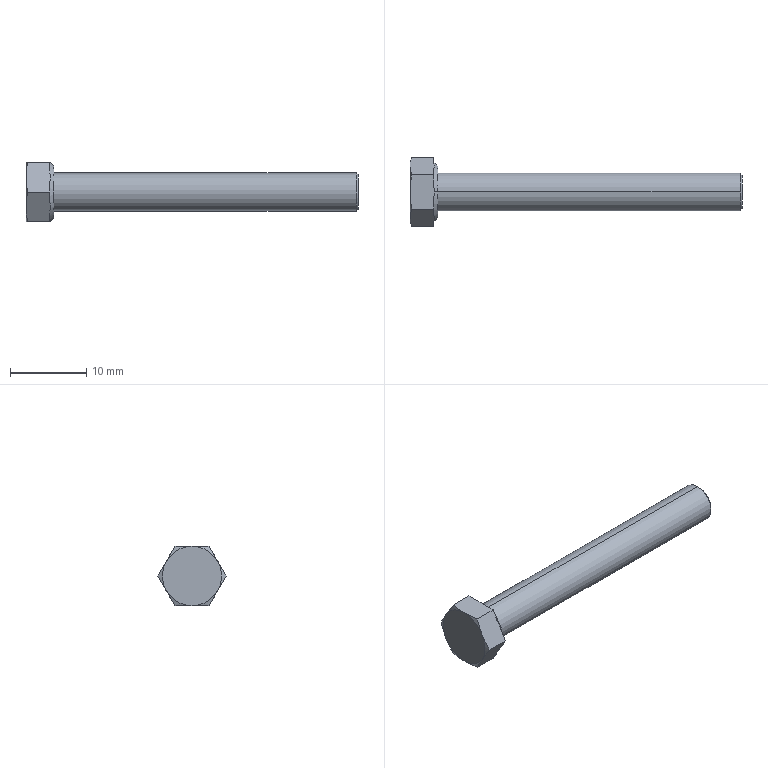Part | SolidWorks | features RevCut 3, Boss 1, Chamfer 1, Extrusion 1, Fillet 1, LPattern 1 | 1 solid | 27 faces | box 43.65 x 8.984 x 7.78 mm | volume 971.133 mm3 | plane 15 | cone 10 | cylinder 2 | commonest cylinder face diameters 5 x2
STEP:
#1=CARTESIAN_POINT('',(43.65,0.,-2.25));
#2=VERTEX_POINT('',#1);
#3=CARTESIAN_POINT('',(43.65,0.,2.25));
#4=VERTEX_POINT('',#3);
#5=CARTESIAN_POINT('',(43.65,0.,0.));
#6=DIRECTION('',(1.,0.,0.));
#7=DIRECTION('',(0.,0.,-1.));
#8=AXIS2_PLACEMENT_3D('',#5,#6,#7);
#9=CIRCLE('',#8,2.25);
#10=EDGE_CURVE('',#2,#4,#9,.T.);
#11=ORIENTED_EDGE('',*,*,#10,.F.);
#12=CARTESIAN_POINT('',(43.4,0.,-2.5));
#13=VERTEX_POINT('',#12);
#14=CARTESIAN_POINT('',(43.65,0.,-2.25));
#15=DIRECTION('',(-0.7071,0.,-0.7071));
#16=VECTOR('',#15,1000.);
#17=LINE('',#14,#16);
#18=EDGE_CURVE('',#2,#13,#17,.T.);
#19=ORIENTED_EDGE('',*,*,#18,.T.);
#20=CARTESIAN_POINT('',(43.4,0.,2.5));
#21=VERTEX_POINT('',#20);
#22=CARTESIAN_POINT('',(43.4,0.,0.));
#23=DIRECTION('',(-1.,0.,0.));
#24=DIRECTION('',(0.,0.,-1.));
#25=AXIS2_PLACEMENT_3D('',#22,#23,#24);
#26=CIRCLE('',#25,2.5);
#27=EDGE_CURVE('',#21,#13,#26,.T.);
#28=ORIENTED_EDGE('',*,*,#27,.F.);
#29=CARTESIAN_POINT('',(43.65,0.,2.25));
#30=DIRECTION('',(-0.7071,0.,0.7071));
#31=VECTOR('',#30,1000.);
#32=LINE('',#29,#31);
#33=EDGE_CURVE('',#4,#21,#32,.T.);
#34=ORIENTED_EDGE('',*,*,#33,.F.);
#35=EDGE_LOOP('',(#11,#19,#28,#34));
#36=FACE_OUTER_BOUND('',#35,.T.);
#37=CARTESIAN_POINT('',(43.65,0.,0.));
#38=DIRECTION('',(-1.,0.,0.));
#39=DIRECTION('',(0.,0.,1.));
#40=AXIS2_PLACEMENT_3D('',#37,#38,#39);
#41=CONICAL_SURFACE('',#40,2.25,0.7854);
#42=ADVANCED_FACE('',(#36),#41,.T.);
#43=ORIENTED_EDGE('',*,*,#27,.T.);
#44=CARTESIAN_POINT('',(3.65,0.,-2.5));
#45=VERTEX_POINT('',#44);
#46=CARTESIAN_POINT('',(43.65,0.,-2.5));
#47=DIRECTION('',(-1.,0.,0.));
#48=VECTOR('',#47,1000.);
#49=LINE('',#46,#48);
#50=EDGE_CURVE('',#13,#45,#49,.T.);
#51=ORIENTED_EDGE('',*,*,#50,.T.);
#52=CARTESIAN_POINT('',(3.65,0.,2.5));
#53=VERTEX_POINT('',#52);
#54=CARTESIAN_POINT('',(3.65,0.,0.));
#55=DIRECTION('',(1.,0.,0.));
#56=DIRECTION('',(0.,0.,-1.));
#57=AXIS2_PLACEMENT_3D('',#54,#55,#56);
#58=CIRCLE('',#57,2.5);
#59=EDGE_CURVE('',#45,#53,#58,.T.);
#60=ORIENTED_EDGE('',*,*,#59,.T.);
#61=CARTESIAN_POINT('',(43.65,0.,2.5));
#62=DIRECTION('',(-1.,0.,0.));
#63=VECTOR('',#62,1000.);
#64=LINE('',#61,#63);
#65=EDGE_CURVE('',#21,#53,#64,.T.);
#66=ORIENTED_EDGE('',*,*,#65,.F.);
#67=EDGE_LOOP('',(#43,#51,#60,#66));
#68=FACE_OUTER_BOUND('',#67,.T.);
#69=CARTESIAN_POINT('',(43.65,0.,0.));
#70=DIRECTION('',(-1.,0.,0.));
#71=DIRECTION('',(0.,0.,1.));
#72=AXIS2_PLACEMENT_3D('',#69,#70,#71);
#73=CYLINDRICAL_SURFACE('',#72,2.5);
#74=ADVANCED_FACE('',(#68),#73,.T.);
#75=CARTESIAN_POINT('',(3.65,0.,3.44));
#76=VERTEX_POINT('',#75);
#77=CARTESIAN_POINT('',(3.65,0.,-3.44));
#78=VERTEX_POINT('',#77);
#79=CARTESIAN_POINT('',(3.65,0.,0.));
#80=DIRECTION('',(-1.,0.,0.));
#81=DIRECTION('',(0.,0.,1.));
#82=AXIS2_PLACEMENT_3D('',#79,#80,#81);
#83=CIRCLE('',#82,3.44);
#84=EDGE_CURVE('',#76,#78,#83,.T.);
#85=ORIENTED_EDGE('',*,*,#84,.T.);
#86=CARTESIAN_POINT('',(3.2,0.,-3.89));
#87=VERTEX_POINT('',#86);
#88=CARTESIAN_POINT('',(3.15,0.,-3.94));
#89=DIRECTION('',(-0.7071,0.,-0.7071));
#90=VECTOR('',#89,1000.);
#91=LINE('',#88,#90);
#92=EDGE_CURVE('',#78,#87,#91,.T.);
#93=ORIENTED_EDGE('',*,*,#92,.T.);
#94=CARTESIAN_POINT('',(3.15,0.6257,-3.89));
#95=VERTEX_POINT('',#94);
#96=CARTESIAN_POINT('',(3.2,0.,-3.89));
#97=CARTESIAN_POINT('',(3.2,0.2088,-3.89));
#98=CARTESIAN_POINT('',(3.183,0.4174,-3.89));
#99=CARTESIAN_POINT('',(3.15,0.6257,-3.89));
#100=B_SPLINE_CURVE_WITH_KNOTS('',3,(#96,#97,#98,#99),.UNSPECIFIED.,.F.,.F.,(4,4),(0.008837,0.009463),.UNSPECIFIED.);
#101=EDGE_CURVE('',#87,#95,#100,.T.);
#102=ORIENTED_EDGE('',*,*,#101,.T.);
#103=CARTESIAN_POINT('',(3.15,3.056,-2.487));
#104=VERTEX_POINT('',#103);
#105=CARTESIAN_POINT('',(3.15,0.,0.));
#106=DIRECTION('',(-1.,0.,0.));
#107=DIRECTION('',(0.,0.,1.));
#108=AXIS2_PLACEMENT_3D('',#105,#106,#107);
#109=CIRCLE('',#108,3.94);
#110=EDGE_CURVE('',#104,#95,#109,.T.);
#111=ORIENTED_EDGE('',*,*,#110,.F.);
#112=CARTESIAN_POINT('',(3.15,3.682,-1.403));
#113=VERTEX_POINT('',#112);
#114=CARTESIAN_POINT('',(3.15,3.056,-2.487));
#115=CARTESIAN_POINT('',(3.216,3.265,-2.126));
#116=CARTESIAN_POINT('',(3.216,3.473,-1.764));
#117=CARTESIAN_POINT('',(3.15,3.682,-1.403));
#118=B_SPLINE_CURVE_WITH_KNOTS('',3,(#114,#115,#116,#117),.UNSPECIFIED.,.F.,.F.,(4,4),(0.000001258,0.001253),.UNSPECIFIED.);
#119=EDGE_CURVE('',#104,#113,#118,.T.);
#120=ORIENTED_EDGE('',*,*,#119,.T.);
#121=CARTESIAN_POINT('',(3.15,3.682,1.403));
#122=VERTEX_POINT('',#121);
#123=CARTESIAN_POINT('',(3.15,0.,0.));
#124=DIRECTION('',(-1.,0.,0.));
#125=DIRECTION('',(0.,0.,1.));
#126=AXIS2_PLACEMENT_3D('',#123,#124,#125);
#127=CIRCLE('',#126,3.94);
#128=EDGE_CURVE('',#122,#113,#127,.T.);
#129=ORIENTED_EDGE('',*,*,#128,.F.);
#130=CARTESIAN_POINT('',(3.15,3.056,2.487));
#131=VERTEX_POINT('',#130);
#132=CARTESIAN_POINT('',(3.15,3.682,1.403));
#133=CARTESIAN_POINT('',(3.216,3.473,1.764));
#134=CARTESIAN_POINT('',(3.216,3.265,2.126));
#135=CARTESIAN_POINT('',(3.15,3.056,2.487));
#136=B_SPLINE_CURVE_WITH_KNOTS('',3,(#132,#133,#134,#135),.UNSPECIFIED.,.F.,.F.,(4,4),(0.000001258,0.001253),.UNSPECIFIED.);
#137=EDGE_CURVE('',#122,#131,#136,.T.);
#138=ORIENTED_EDGE('',*,*,#137,.T.);
#139=CARTESIAN_POINT('',(3.15,0.6257,3.89));
#140=VERTEX_POINT('',#139);
#141=CARTESIAN_POINT('',(3.15,0.,0.));
#142=DIRECTION('',(-1.,0.,0.));
#143=DIRECTION('',(0.,0.,1.));
#144=AXIS2_PLACEMENT_3D('',#141,#142,#143);
#145=CIRCLE('',#144,3.94);
#146=EDGE_CURVE('',#140,#131,#145,.T.);
#147=ORIENTED_EDGE('',*,*,#146,.F.);
#148=CARTESIAN_POINT('',(3.2,0.,3.89));
#149=VERTEX_POINT('',#148);
#150=CARTESIAN_POINT('',(3.15,0.6257,3.89));
#151=CARTESIAN_POINT('',(3.183,0.4208,3.89));
#152=CARTESIAN_POINT('',(3.2,0.2096,3.89));
#153=CARTESIAN_POINT('',(3.2,0.,3.89));
#154=B_SPLINE_CURVE_WITH_KNOTS('',3,(#150,#151,#152,#153),.UNSPECIFIED.,.F.,.F.,(4,4),(0.001763,0.00238),.UNSPECIFIED.);
#155=EDGE_CURVE('',#140,#149,#154,.T.);
#156=ORIENTED_EDGE('',*,*,#155,.T.);
#157=CARTESIAN_POINT('',(3.15,0.,3.94));
#158=DIRECTION('',(-0.7071,0.,0.7071));
#159=VECTOR('',#158,1000.);
#160=LINE('',#157,#159);
#161=EDGE_CURVE('',#76,#149,#160,.T.);
#162=ORIENTED_EDGE('',*,*,#161,.F.);
#163=EDGE_LOOP('',(#85,#93,#102,#111,#120,#129,#138,#147,#156,#162));
#164=FACE_OUTER_BOUND('',#163,.T.);
#165=CARTESIAN_POINT('',(3.15,0.,0.));
#166=DIRECTION('',(-1.,0.,0.));
#167=DIRECTION('',(0.,0.,1.));
#168=AXIS2_PLACEMENT_3D('',#165,#166,#167);
#169=CONICAL_SURFACE('',#168,3.94,0.7854);
#170=ADVANCED_FACE('',(#164),#169,.T.);
#171=ORIENTED_EDGE('',*,*,#84,.F.);
#172=CARTESIAN_POINT('',(3.65,0.,0.));
#173=DIRECTION('',(-1.,0.,0.));
#174=DIRECTION('',(0.,0.,1.));
#175=AXIS2_PLACEMENT_3D('',#172,#173,#174);
#176=CIRCLE('',#175,3.44);
#177=EDGE_CURVE('',#78,#76,#176,.T.);
#178=ORIENTED_EDGE('',*,*,#177,.F.);
#179=EDGE_LOOP('',(#171,#178));
#180=FACE_OUTER_BOUND('',#179,.T.);
#181=CARTESIAN_POINT('',(3.65,0.,0.));
#182=DIRECTION('',(1.,0.,0.));
#183=DIRECTION('',(0.,0.,-1.));
#184=AXIS2_PLACEMENT_3D('',#181,#182,#183);
#185=CIRCLE('',#184,2.5);
#186=EDGE_CURVE('',#53,#45,#185,.T.);
#187=ORIENTED_EDGE('',*,*,#186,.F.);
#188=ORIENTED_EDGE('',*,*,#59,.F.);
#189=EDGE_LOOP('',(#187,#188));
#190=FACE_BOUND('',#189,.T.);
#191=CARTESIAN_POINT('',(3.65,-2.246,-3.89));
#192=DIRECTION('',(1.,0.,0.));
#193=DIRECTION('',(0.,0.,-1.));
#194=AXIS2_PLACEMENT_3D('',#191,#192,#193);
#195=PLANE('',#194);
#196=ADVANCED_FACE('',(#180,#190),#195,.T.);
#197=CARTESIAN_POINT('',(0.219,-2.246,-3.89));
#198=VERTEX_POINT('',#197);
#199=CARTESIAN_POINT('',(0.,-3.369,-1.945));
#200=VERTEX_POINT('',#199);
#201=CARTESIAN_POINT('',(0.219,-2.246,-3.89));
#202=CARTESIAN_POINT('',(0.08279,-2.62,-3.242));
#203=CARTESIAN_POINT('',(0.,-2.995,-2.593));
#204=CARTESIAN_POINT('',(0.,-3.369,-1.945));
#205=B_SPLINE_CURVE_WITH_KNOTS('',3,(#201,#202,#203,#204),.UNSPECIFIED.,.F.,.F.,(4,4),(0.000000231,0.002246),.UNSPECIFIED.);
#206=EDGE_CURVE('',#198,#200,#205,.T.);
#207=ORIENTED_EDGE('',*,*,#206,.F.);
#208=CARTESIAN_POINT('',(3.15,-2.246,-3.89));
#209=VERTEX_POINT('',#208);
#210=CARTESIAN_POINT('',(3.65,-2.246,-3.89));
#211=DIRECTION('',(-1.,0.,0.));
#212=VECTOR('',#211,1000.);
#213=LINE('',#210,#212);
#214=EDGE_CURVE('',#209,#198,#213,.T.);
#215=ORIENTED_EDGE('',*,*,#214,.F.);
#216=CARTESIAN_POINT('',(3.15,-3.056,-2.487));
#217=VERTEX_POINT('',#216);
#218=CARTESIAN_POINT('',(3.15,-4.492,0.));
#219=DIRECTION('',(0.,0.5,-0.866));
#220=VECTOR('',#219,1000.);
#221=LINE('',#218,#220);
#222=EDGE_CURVE('',#217,#209,#221,.T.);
#223=ORIENTED_EDGE('',*,*,#222,.F.);
#224=CARTESIAN_POINT('',(3.15,-3.682,-1.403));
#225=VERTEX_POINT('',#224);
#226=CARTESIAN_POINT('',(3.15,-3.682,-1.403));
#227=CARTESIAN_POINT('',(3.216,-3.473,-1.764));
#228=CARTESIAN_POINT('',(3.216,-3.265,-2.126));
#229=CARTESIAN_POINT('',(3.15,-3.056,-2.487));
#230=B_SPLINE_CURVE_WITH_KNOTS('',3,(#226,#227,#228,#229),.UNSPECIFIED.,.F.,.F.,(4,4),(0.000001258,0.001253),.UNSPECIFIED.);
#231=EDGE_CURVE('',#225,#217,#230,.T.);
#232=ORIENTED_EDGE('',*,*,#231,.F.);
#233=CARTESIAN_POINT('',(3.15,-4.492,0.));
#234=VERTEX_POINT('',#233);
#235=CARTESIAN_POINT('',(3.15,-4.492,0.));
#236=DIRECTION('',(0.,0.5,-0.866));
#237=VECTOR('',#236,1000.);
#238=LINE('',#235,#237);
#239=EDGE_CURVE('',#234,#225,#238,.T.);
#240=ORIENTED_EDGE('',*,*,#239,.F.);
#241=CARTESIAN_POINT('',(0.219,-4.492,0.));
#242=VERTEX_POINT('',#241);
#243=CARTESIAN_POINT('',(3.65,-4.492,0.));
#244=DIRECTION('',(-1.,0.,0.));
#245=VECTOR('',#244,1000.);
#246=LINE('',#243,#245);
#247=EDGE_CURVE('',#234,#242,#246,.T.);
#248=ORIENTED_EDGE('',*,*,#247,.T.);
#249=CARTESIAN_POINT('',(0.,-3.369,-1.945));
#250=CARTESIAN_POINT('',(0.,-3.743,-1.297));
#251=CARTESIAN_POINT('',(0.08279,-4.117,-0.6483));
#252=CARTESIAN_POINT('',(0.219,-4.492,0.));
#253=B_SPLINE_CURVE_WITH_KNOTS('',3,(#249,#250,#251,#252),.UNSPECIFIED.,.F.,.F.,(4,4),(0.002246,0.004492),.UNSPECIFIED.);
#254=EDGE_CURVE('',#200,#242,#253,.T.);
#255=ORIENTED_EDGE('',*,*,#254,.F.);
#256=EDGE_LOOP('',(#207,#215,#223,#232,#240,#248,#255));
#257=FACE_OUTER_BOUND('',#256,.T.);
#258=CARTESIAN_POINT('',(3.65,-4.492,0.));
#259=DIRECTION('',(0.,0.866,0.5));
#260=DIRECTION('',(0.,-0.5,0.866));
#261=AXIS2_PLACEMENT_3D('',#258,#259,#260);
#262=PLANE('',#261);
#263=ADVANCED_FACE('',(#257),#262,.F.);
#264=CARTESIAN_POINT('',(0.219,2.246,-3.89));
#265=VERTEX_POINT('',#264);
#266=CARTESIAN_POINT('',(0.,0.,-3.89));
#267=VERTEX_POINT('',#266);
#268=CARTESIAN_POINT('',(0.219,2.246,-3.89));
#269=CARTESIAN_POINT('',(0.08316,1.499,-3.89));
#270=CARTESIAN_POINT('',(0.,0.7502,-3.89));
#271=CARTESIAN_POINT('',(0.,0.,-3.89));
#272=B_SPLINE_CURVE_WITH_KNOTS('',3,(#268,#269,#270,#271),.UNSPECIFIED.,.F.,.F.,(4,4),(0.008099,0.01036),.UNSPECIFIED.);
#273=EDGE_CURVE('',#265,#267,#272,.T.);
#274=ORIENTED_EDGE('',*,*,#273,.F.);
#275=CARTESIAN_POINT('',(3.15,2.246,-3.89));
#276=VERTEX_POINT('',#275);
#277=CARTESIAN_POINT('',(3.65,2.246,-3.89));
#278=DIRECTION('',(-1.,0.,0.));
#279=VECTOR('',#278,1000.);
#280=LINE('',#277,#279);
#281=EDGE_CURVE('',#276,#265,#280,.T.);
#282=ORIENTED_EDGE('',*,*,#281,.F.);
#283=CARTESIAN_POINT('',(3.15,-2.246,-3.89));
#284=DIRECTION('',(0.,1.,0.));
#285=VECTOR('',#284,1000.);
#286=LINE('',#283,#285);
#287=EDGE_CURVE('',#95,#276,#286,.T.);
#288=ORIENTED_EDGE('',*,*,#287,.F.);
#289=ORIENTED_EDGE('',*,*,#101,.F.);
#290=CARTESIAN_POINT('',(3.15,-0.6257,-3.89));
#291=VERTEX_POINT('',#290);
#292=CARTESIAN_POINT('',(3.15,-0.6257,-3.89));
#293=CARTESIAN_POINT('',(3.183,-0.4181,-3.89));
#294=CARTESIAN_POINT('',(3.2,-0.2084,-3.89));
#295=CARTESIAN_POINT('',(3.2,0.,-3.89));
#296=B_SPLINE_CURVE_WITH_KNOTS('',3,(#292,#293,#294,#295),.UNSPECIFIED.,.F.,.F.,(4,4),(0.008211,0.008837),.UNSPECIFIED.);
#297=EDGE_CURVE('',#291,#87,#296,.T.);
#298=ORIENTED_EDGE('',*,*,#297,.F.);
#299=CARTESIAN_POINT('',(3.15,-2.246,-3.89));
#300=DIRECTION('',(0.,1.,0.));
#301=VECTOR('',#300,1000.);
#302=LINE('',#299,#301);
#303=EDGE_CURVE('',#209,#291,#302,.T.);
#304=ORIENTED_EDGE('',*,*,#303,.F.);
#305=ORIENTED_EDGE('',*,*,#214,.T.);
#306=CARTESIAN_POINT('',(0.,0.,-3.89));
#307=CARTESIAN_POINT('',(0.,-0.374,-3.89));
#308=CARTESIAN_POINT('',(0.02,-0.7484,-3.89));
#309=CARTESIAN_POINT('',(0.09569,-1.498,-3.89));
#310=CARTESIAN_POINT('',(0.1514,-1.874,-3.89));
#311=CARTESIAN_POINT('',(0.219,-2.246,-3.89));
#312=B_SPLINE_CURVE_WITH_KNOTS('',3,(#306,#307,#308,#309,#310,#311),.UNSPECIFIED.,.F.,.F.,(4,2,4),(0.01036,0.01149,0.01262),.UNSPECIFIED.);
#313=EDGE_CURVE('',#267,#198,#312,.T.);
#314=ORIENTED_EDGE('',*,*,#313,.F.);
#315=EDGE_LOOP('',(#274,#282,#288,#289,#298,#304,#305,#314));
#316=FACE_OUTER_BOUND('',#315,.T.);
#317=CARTESIAN_POINT('',(3.65,-2.246,-3.89));
#318=DIRECTION('',(0.,0.,1.));
#319=DIRECTION('',(0.,-1.,0.));
#320=AXIS2_PLACEMENT_3D('',#317,#318,#319);
#321=PLANE('',#320);
#322=ADVANCED_FACE('',(#316),#321,.F.);
#323=CARTESIAN_POINT('',(0.219,4.492,0.));
#324=VERTEX_POINT('',#323);
#325=CARTESIAN_POINT('',(0.,3.369,-1.945));
#326=VERTEX_POINT('',#325);
#327=CARTESIAN_POINT('',(0.219,4.492,0.));
#328=CARTESIAN_POINT('',(0.08279,4.117,-0.6483));
#329=CARTESIAN_POINT('',(0.,3.743,-1.297));
#330=CARTESIAN_POINT('',(0.,3.369,-1.945));
#331=B_SPLINE_CURVE_WITH_KNOTS('',3,(#327,#328,#329,#330),.UNSPECIFIED.,.F.,.F.,(4,4),(0.000000231,0.002246),.UNSPECIFIED.);
#332=EDGE_CURVE('',#324,#326,#331,.T.);
#333=ORIENTED_EDGE('',*,*,#332,.F.);
#334=CARTESIAN_POINT('',(3.15,4.492,0.));
#335=VERTEX_POINT('',#334);
#336=CARTESIAN_POINT('',(3.65,4.492,0.));
#337=DIRECTION('',(-1.,0.,0.));
#338=VECTOR('',#337,1000.);
#339=LINE('',#336,#338);
#340=EDGE_CURVE('',#335,#324,#339,.T.);
#341=ORIENTED_EDGE('',*,*,#340,.F.);
#342=CARTESIAN_POINT('',(3.15,2.246,-3.89));
#343=DIRECTION('',(0.,0.5,0.866));
#344=VECTOR('',#343,1000.);
#345=LINE('',#342,#344);
#346=EDGE_CURVE('',#113,#335,#345,.T.);
#347=ORIENTED_EDGE('',*,*,#346,.F.);
#348=ORIENTED_EDGE('',*,*,#119,.F.);
#349=CARTESIAN_POINT('',(3.15,2.246,-3.89));
#350=DIRECTION('',(0.,0.5,0.866));
#351=VECTOR('',#350,1000.);
#352=LINE('',#349,#351);
#353=EDGE_CURVE('',#276,#104,#352,.T.);
#354=ORIENTED_EDGE('',*,*,#353,.F.);
#355=ORIENTED_EDGE('',*,*,#281,.T.);
#356=CARTESIAN_POINT('',(0.,3.369,-1.945));
#357=CARTESIAN_POINT('',(0.,2.995,-2.593));
#358=CARTESIAN_POINT('',(0.08279,2.62,-3.242));
#359=CARTESIAN_POINT('',(0.219,2.246,-3.89));
#360=B_SPLINE_CURVE_WITH_KNOTS('',3,(#356,#357,#358,#359),.UNSPECIFIED.,.F.,.F.,(4,4),(0.002246,0.004492),.UNSPECIFIED.);
#361=EDGE_CURVE('',#326,#265,#360,.T.);
#362=ORIENTED_EDGE('',*,*,#361,.F.);
#363=EDGE_LOOP('',(#333,#341,#347,#348,#354,#355,#362));
#364=FACE_OUTER_BOUND('',#363,.T.);
#365=CARTESIAN_POINT('',(3.65,2.246,-3.89));
#366=DIRECTION('',(0.,-0.866,0.5));
#367=DIRECTION('',(0.,-0.5,-0.866));
#368=AXIS2_PLACEMENT_3D('',#365,#366,#367);
#369=PLANE('',#368);
#370=ADVANCED_FACE('',(#364),#369,.F.);
#371=CARTESIAN_POINT('',(0.219,2.246,3.89));
#372=VERTEX_POINT('',#371);
#373=CARTESIAN_POINT('',(0.,3.369,1.945));
#374=VERTEX_POINT('',#373);
#375=CARTESIAN_POINT('',(0.219,2.246,3.89));
#376=CARTESIAN_POINT('',(0.08279,2.62,3.242));
#377=CARTESIAN_POINT('',(0.,2.995,2.593));
#378=CARTESIAN_POINT('',(0.,3.369,1.945));
#379=B_SPLINE_CURVE_WITH_KNOTS('',3,(#375,#376,#377,#378),.UNSPECIFIED.,.F.,.F.,(4,4),(0.000000231,0.002246),.UNSPECIFIED.);
#380=EDGE_CURVE('',#372,#374,#379,.T.);
#381=ORIENTED_EDGE('',*,*,#380,.F.);
#382=CARTESIAN_POINT('',(3.15,2.246,3.89));
#383=VERTEX_POINT('',#382);
#384=CARTESIAN_POINT('',(3.65,2.246,3.89));
#385=DIRECTION('',(-1.,0.,0.));
#386=VECTOR('',#385,1000.);
#387=LINE('',#384,#386);
#388=EDGE_CURVE('',#383,#372,#387,.T.);
#389=ORIENTED_EDGE('',*,*,#388,.F.);
#390=CARTESIAN_POINT('',(3.15,4.492,0.));
#391=DIRECTION('',(0.,-0.5,0.866));
#392=VECTOR('',#391,1000.);
#393=LINE('',#390,#392);
#394=EDGE_CURVE('',#131,#383,#393,.T.);
#395=ORIENTED_EDGE('',*,*,#394,.F.);
#396=ORIENTED_EDGE('',*,*,#137,.F.);
#397=CARTESIAN_POINT('',(3.15,4.492,0.));
#398=DIRECTION('',(0.,-0.5,0.866));
#399=VECTOR('',#398,1000.);
#400=LINE('',#397,#399);
#401=EDGE_CURVE('',#335,#122,#400,.T.);
#402=ORIENTED_EDGE('',*,*,#401,.F.);
#403=ORIENTED_EDGE('',*,*,#340,.T.);
#404=CARTESIAN_POINT('',(0.,3.369,1.945));
#405=CARTESIAN_POINT('',(0.,3.743,1.297));
#406=CARTESIAN_POINT('',(0.08279,4.117,0.6483));
#407=CARTESIAN_POINT('',(0.219,4.492,0.));
#408=B_SPLINE_CURVE_WITH_KNOTS('',3,(#404,#405,#406,#407),.UNSPECIFIED.,.F.,.F.,(4,4),(0.002246,0.004492),.UNSPECIFIED.);
#409=EDGE_CURVE('',#374,#324,#408,.T.);
#410=ORIENTED_EDGE('',*,*,#409,.F.);
#411=EDGE_LOOP('',(#381,#389,#395,#396,#402,#403,#410));
#412=FACE_OUTER_BOUND('',#411,.T.);
#413=CARTESIAN_POINT('',(3.65,4.492,0.));
#414=DIRECTION('',(0.,-0.866,-0.5));
#415=DIRECTION('',(0.,0.5,-0.866));
#416=AXIS2_PLACEMENT_3D('',#413,#414,#415);
#417=PLANE('',#416);
#418=ADVANCED_FACE('',(#412),#417,.F.);
#419=CARTESIAN_POINT('',(0.219,-2.246,3.89));
#420=VERTEX_POINT('',#419);
#421=CARTESIAN_POINT('',(0.,0.,3.89));
#422=VERTEX_POINT('',#421);
#423=CARTESIAN_POINT('',(0.219,-2.246,3.89));
#424=CARTESIAN_POINT('',(0.1514,-1.874,3.89));
#425=CARTESIAN_POINT('',(0.09569,-1.498,3.89));
#426=CARTESIAN_POINT('',(0.02,-0.7484,3.89));
#427=CARTESIAN_POINT('',(0.,-0.374,3.89));
#428=CARTESIAN_POINT('',(0.,0.,3.89));
#429=B_SPLINE_CURVE_WITH_KNOTS('',3,(#423,#424,#425,#426,#427,#428),.UNSPECIFIED.,.F.,.F.,(4,2,4),(0.003821,0.004952,0.006084),.UNSPECIFIED.);
#430=EDGE_CURVE('',#420,#422,#429,.T.);
#431=ORIENTED_EDGE('',*,*,#430,.F.);
#432=CARTESIAN_POINT('',(3.15,-2.246,3.89));
#433=VERTEX_POINT('',#432);
#434=CARTESIAN_POINT('',(3.65,-2.246,3.89));
#435=DIRECTION('',(-1.,0.,0.));
#436=VECTOR('',#435,1000.);
#437=LINE('',#434,#436);
#438=EDGE_CURVE('',#433,#420,#437,.T.);
#439=ORIENTED_EDGE('',*,*,#438,.F.);
#440=CARTESIAN_POINT('',(3.15,-0.6257,3.89));
#441=VERTEX_POINT('',#440);
#442=CARTESIAN_POINT('',(3.15,2.246,3.89));
#443=DIRECTION('',(0.,-1.,0.));
#444=VECTOR('',#443,1000.);
#445=LINE('',#442,#444);
#446=EDGE_CURVE('',#441,#433,#445,.T.);
#447=ORIENTED_EDGE('',*,*,#446,.F.);
#448=CARTESIAN_POINT('',(3.2,0.,3.89));
#449=CARTESIAN_POINT('',(3.2,-0.2092,3.89));
#450=CARTESIAN_POINT('',(3.183,-0.4189,3.89));
#451=CARTESIAN_POINT('',(3.15,-0.6257,3.89));
#452=B_SPLINE_CURVE_WITH_KNOTS('',3,(#448,#449,#450,#451),.UNSPECIFIED.,.F.,.F.,(4,4),(0.00238,0.002995),.UNSPECIFIED.);
#453=EDGE_CURVE('',#149,#441,#452,.T.);
#454=ORIENTED_EDGE('',*,*,#453,.F.);
#455=ORIENTED_EDGE('',*,*,#155,.F.);
#456=CARTESIAN_POINT('',(3.15,2.246,3.89));
#457=DIRECTION('',(0.,-1.,0.));
#458=VECTOR('',#457,1000.);
#459=LINE('',#456,#458);
#460=EDGE_CURVE('',#383,#140,#459,.T.);
#461=ORIENTED_EDGE('',*,*,#460,.F.);
#462=ORIENTED_EDGE('',*,*,#388,.T.);
#463=CARTESIAN_POINT('',(0.,0.,3.89));
#464=CARTESIAN_POINT('',(0.,0.7502,3.89));
#465=CARTESIAN_POINT('',(0.08316,1.499,3.89));
#466=CARTESIAN_POINT('',(0.219,2.246,3.89));
#467=B_SPLINE_CURVE_WITH_KNOTS('',3,(#463,#464,#465,#466),.UNSPECIFIED.,.F.,.F.,(4,4),(0.006084,0.008354),.UNSPECIFIED.);
#468=EDGE_CURVE('',#422,#372,#467,.T.);
#469=ORIENTED_EDGE('',*,*,#468,.F.);
#470=EDGE_LOOP('',(#431,#439,#447,#454,#455,#461,#462,#469));
#471=FACE_OUTER_BOUND('',#470,.T.);
#472=CARTESIAN_POINT('',(3.65,2.246,3.89));
#473=DIRECTION('',(0.,0.,-1.));
#474=DIRECTION('',(-1.,0.,0.));
#475=AXIS2_PLACEMENT_3D('',#472,#473,#474);
#476=PLANE('',#475);
#477=ADVANCED_FACE('',(#471),#476,.F.);
#478=CARTESIAN_POINT('',(0.,-3.369,1.945));
#479=VERTEX_POINT('',#478);
#480=CARTESIAN_POINT('',(0.219,-4.492,0.));
#481=CARTESIAN_POINT('',(0.08279,-4.117,0.6483));
#482=CARTESIAN_POINT('',(0.,-3.743,1.297));
#483=CARTESIAN_POINT('',(0.,-3.369,1.945));
#484=B_SPLINE_CURVE_WITH_KNOTS('',3,(#480,#481,#482,#483),.UNSPECIFIED.,.F.,.F.,(4,4),(0.000000231,0.002246),.UNSPECIFIED.);
#485=EDGE_CURVE('',#242,#479,#484,.T.);
#486=ORIENTED_EDGE('',*,*,#485,.F.);
#487=ORIENTED_EDGE('',*,*,#247,.F.);
#488=CARTESIAN_POINT('',(3.15,-3.682,1.403));
#489=VERTEX_POINT('',#488);
#490=CARTESIAN_POINT('',(3.15,-2.246,3.89));
#491=DIRECTION('',(0.,-0.5,-0.866));
#492=VECTOR('',#491,1000.);
#493=LINE('',#490,#492);
#494=EDGE_CURVE('',#489,#234,#493,.T.);
#495=ORIENTED_EDGE('',*,*,#494,.F.);
#496=CARTESIAN_POINT('',(3.15,-3.056,2.487));
#497=VERTEX_POINT('',#496);
#498=CARTESIAN_POINT('',(3.15,-3.056,2.487));
#499=CARTESIAN_POINT('',(3.216,-3.265,2.126));
#500=CARTESIAN_POINT('',(3.216,-3.473,1.764));
#501=CARTESIAN_POINT('',(3.15,-3.682,1.403));
#502=B_SPLINE_CURVE_WITH_KNOTS('',3,(#498,#499,#500,#501),.UNSPECIFIED.,.F.,.F.,(4,4),(0.000001258,0.001253),.UNSPECIFIED.);
#503=EDGE_CURVE('',#497,#489,#502,.T.);
#504=ORIENTED_EDGE('',*,*,#503,.F.);
#505=CARTESIAN_POINT('',(3.15,-2.246,3.89));
#506=DIRECTION('',(0.,-0.5,-0.866));
#507=VECTOR('',#506,1000.);
#508=LINE('',#505,#507);
#509=EDGE_CURVE('',#433,#497,#508,.T.);
#510=ORIENTED_EDGE('',*,*,#509,.F.);
#511=ORIENTED_EDGE('',*,*,#438,.T.);
#512=CARTESIAN_POINT('',(0.,-3.369,1.945));
#513=CARTESIAN_POINT('',(0.,-2.995,2.593));
#514=CARTESIAN_POINT('',(0.08279,-2.62,3.242));
#515=CARTESIAN_POINT('',(0.219,-2.246,3.89));
#516=B_SPLINE_CURVE_WITH_KNOTS('',3,(#512,#513,#514,#515),.UNSPECIFIED.,.F.,.F.,(4,4),(0.002246,0.004492),.UNSPECIFIED.);
#517=EDGE_CURVE('',#479,#420,#516,.T.);
#518=ORIENTED_EDGE('',*,*,#517,.F.);
#519=EDGE_LOOP('',(#486,#487,#495,#504,#510,#511,#518));
#520=FACE_OUTER_BOUND('',#519,.T.);
#521=CARTESIAN_POINT('',(3.65,-2.246,3.89));
#522=DIRECTION('',(0.,0.866,-0.5));
#523=DIRECTION('',(0.,0.5,0.866));
#524=AXIS2_PLACEMENT_3D('',#521,#522,#523);
#525=PLANE('',#524);
#526=ADVANCED_FACE('',(#520),#525,.F.);
#527=ORIENTED_EDGE('',*,*,#222,.T.);
#528=ORIENTED_EDGE('',*,*,#303,.T.);
#529=CARTESIAN_POINT('',(3.15,0.,0.));
#530=DIRECTION('',(-1.,0.,0.));
#531=DIRECTION('',(0.,0.,1.));
#532=AXIS2_PLACEMENT_3D('',#529,#530,#531);
#533=CIRCLE('',#532,3.94);
#534=EDGE_CURVE('',#291,#217,#533,.T.);
#535=ORIENTED_EDGE('',*,*,#534,.T.);
#536=EDGE_LOOP('',(#527,#528,#535));
#537=FACE_OUTER_BOUND('',#536,.T.);
#538=CARTESIAN_POINT('',(3.15,3.94,0.));
#539=DIRECTION('',(1.,0.,0.));
#540=DIRECTION('',(0.,0.,-1.));
#541=AXIS2_PLACEMENT_3D('',#538,#539,#540);
#542=PLANE('',#541);
#543=ADVANCED_FACE('',(#537),#542,.T.);
#544=ORIENTED_EDGE('',*,*,#287,.T.);
#545=ORIENTED_EDGE('',*,*,#353,.T.);
#546=ORIENTED_EDGE('',*,*,#110,.T.);
#547=EDGE_LOOP('',(#544,#545,#546));
#548=FACE_OUTER_BOUND('',#547,.T.);
#549=CARTESIAN_POINT('',(3.15,3.94,0.));
#550=DIRECTION('',(1.,0.,0.));
#551=DIRECTION('',(0.,0.,-1.));
#552=AXIS2_PLACEMENT_3D('',#549,#550,#551);
#553=PLANE('',#552);
#554=ADVANCED_FACE('',(#548),#553,.T.);
#555=ORIENTED_EDGE('',*,*,#346,.T.);
#556=ORIENTED_EDGE('',*,*,#401,.T.);
#557=ORIENTED_EDGE('',*,*,#128,.T.);
#558=EDGE_LOOP('',(#555,#556,#557));
#559=FACE_OUTER_BOUND('',#558,.T.);
#560=CARTESIAN_POINT('',(3.15,3.94,0.));
#561=DIRECTION('',(1.,0.,0.));
#562=DIRECTION('',(0.,0.,-1.));
#563=AXIS2_PLACEMENT_3D('',#560,#561,#562);
#564=PLANE('',#563);
#565=ADVANCED_FACE('',(#559),#564,.T.);
#566=ORIENTED_EDGE('',*,*,#394,.T.);
#567=ORIENTED_EDGE('',*,*,#460,.T.);
#568=ORIENTED_EDGE('',*,*,#146,.T.);
#569=EDGE_LOOP('',(#566,#567,#568));
#570=FACE_OUTER_BOUND('',#569,.T.);
#571=CARTESIAN_POINT('',(3.15,3.94,0.));
#572=DIRECTION('',(1.,0.,0.));
#573=DIRECTION('',(0.,0.,-1.));
#574=AXIS2_PLACEMENT_3D('',#571,#572,#573);
#575=PLANE('',#574);
#576=ADVANCED_FACE('',(#570),#575,.T.);
#577=ORIENTED_EDGE('',*,*,#446,.T.);
#578=ORIENTED_EDGE('',*,*,#509,.T.);
#579=CARTESIAN_POINT('',(3.15,0.,0.));
#580=DIRECTION('',(-1.,0.,0.));
#581=DIRECTION('',(0.,0.,1.));
#582=AXIS2_PLACEMENT_3D('',#579,#580,#581);
#583=CIRCLE('',#582,3.94);
#584=EDGE_CURVE('',#497,#441,#583,.T.);
#585=ORIENTED_EDGE('',*,*,#584,.T.);
#586=EDGE_LOOP('',(#577,#578,#585));
#587=FACE_OUTER_BOUND('',#586,.T.);
#588=CARTESIAN_POINT('',(3.15,3.94,0.));
#589=DIRECTION('',(1.,0.,0.));
#590=DIRECTION('',(0.,0.,-1.));
#591=AXIS2_PLACEMENT_3D('',#588,#589,#590);
#592=PLANE('',#591);
#593=ADVANCED_FACE('',(#587),#592,.T.);
#594=ORIENTED_EDGE('',*,*,#239,.T.);
#595=CARTESIAN_POINT('',(3.15,0.,0.));
#596=DIRECTION('',(-1.,0.,0.));
#597=DIRECTION('',(0.,0.,1.));
#598=AXIS2_PLACEMENT_3D('',#595,#596,#597);
#599=CIRCLE('',#598,3.94);
#600=EDGE_CURVE('',#225,#489,#599,.T.);
#601=ORIENTED_EDGE('',*,*,#600,.T.);
#602=ORIENTED_EDGE('',*,*,#494,.T.);
#603=EDGE_LOOP('',(#594,#601,#602));
#604=FACE_OUTER_BOUND('',#603,.T.);
#605=CARTESIAN_POINT('',(3.15,3.94,0.));
#606=DIRECTION('',(1.,0.,0.));
#607=DIRECTION('',(0.,0.,-1.));
#608=AXIS2_PLACEMENT_3D('',#605,#606,#607);
#609=PLANE('',#608);
#610=ADVANCED_FACE('',(#604),#609,.T.);
#611=ORIENTED_EDGE('',*,*,#92,.F.);
#612=ORIENTED_EDGE('',*,*,#177,.T.);
#613=ORIENTED_EDGE('',*,*,#161,.T.);
#614=ORIENTED_EDGE('',*,*,#453,.T.);
#615=ORIENTED_EDGE('',*,*,#584,.F.);
#616=ORIENTED_EDGE('',*,*,#503,.T.);
#617=ORIENTED_EDGE('',*,*,#600,.F.);
#618=ORIENTED_EDGE('',*,*,#231,.T.);
#619=ORIENTED_EDGE('',*,*,#534,.F.);
#620=ORIENTED_EDGE('',*,*,#297,.T.);
#621=EDGE_LOOP('',(#611,#612,#613,#614,#615,#616,#617,#618,#619,#620));
#622=FACE_OUTER_BOUND('',#621,.T.);
#623=CARTESIAN_POINT('',(3.15,0.,0.));
#624=DIRECTION('',(-1.,0.,0.));
#625=DIRECTION('',(0.,0.,1.));
#626=AXIS2_PLACEMENT_3D('',#623,#624,#625);
#627=CONICAL_SURFACE('',#626,3.94,0.7854);
#628=ADVANCED_FACE('',(#622),#627,.T.);
#629=ORIENTED_EDGE('',*,*,#313,.T.);
#630=ORIENTED_EDGE('',*,*,#206,.T.);
#631=CARTESIAN_POINT('',(0.,0.,0.));
#632=DIRECTION('',(1.,0.,0.));
#633=DIRECTION('',(0.,0.,-1.));
#634=AXIS2_PLACEMENT_3D('',#631,#632,#633);
#635=CIRCLE('',#634,3.89);
#636=EDGE_CURVE('',#200,#267,#635,.T.);
#637=ORIENTED_EDGE('',*,*,#636,.T.);
#638=EDGE_LOOP('',(#629,#630,#637));
#639=FACE_OUTER_BOUND('',#638,.T.);
#640=CARTESIAN_POINT('',(0.,0.,0.));
#641=DIRECTION('',(1.,0.,0.));
#642=DIRECTION('',(0.,0.,-1.));
#643=AXIS2_PLACEMENT_3D('',#640,#641,#642);
#644=CONICAL_SURFACE('',#643,3.89,1.222);
#645=ADVANCED_FACE('',(#639),#644,.T.);
#646=ORIENTED_EDGE('',*,*,#254,.T.);
#647=ORIENTED_EDGE('',*,*,#485,.T.);
#648=CARTESIAN_POINT('',(0.,0.,0.));
#649=DIRECTION('',(1.,0.,0.));
#650=DIRECTION('',(0.,0.,-1.));
#651=AXIS2_PLACEMENT_3D('',#648,#649,#650);
#652=CIRCLE('',#651,3.89);
#653=EDGE_CURVE('',#479,#200,#652,.T.);
#654=ORIENTED_EDGE('',*,*,#653,.T.);
#655=EDGE_LOOP('',(#646,#647,#654));
#656=FACE_OUTER_BOUND('',#655,.T.);
#657=CARTESIAN_POINT('',(0.,0.,0.));
#658=DIRECTION('',(1.,0.,0.));
#659=DIRECTION('',(0.,0.,-1.));
#660=AXIS2_PLACEMENT_3D('',#657,#658,#659);
#661=CONICAL_SURFACE('',#660,3.89,1.222);
#662=ADVANCED_FACE('',(#656),#661,.T.);
#663=ORIENTED_EDGE('',*,*,#430,.T.);
#664=CARTESIAN_POINT('',(0.,0.,0.));
#665=DIRECTION('',(1.,0.,0.));
#666=DIRECTION('',(0.,0.,-1.));
#667=AXIS2_PLACEMENT_3D('',#664,#665,#666);
#668=CIRCLE('',#667,3.89);
#669=EDGE_CURVE('',#422,#479,#668,.T.);
#670=ORIENTED_EDGE('',*,*,#669,.T.);
#671=ORIENTED_EDGE('',*,*,#517,.T.);
#672=EDGE_LOOP('',(#663,#670,#671));
#673=FACE_OUTER_BOUND('',#672,.T.);
#674=CARTESIAN_POINT('',(0.,0.,0.));
#675=DIRECTION('',(1.,0.,0.));
#676=DIRECTION('',(0.,0.,-1.));
#677=AXIS2_PLACEMENT_3D('',#674,#675,#676);
#678=CONICAL_SURFACE('',#677,3.89,1.222);
#679=ADVANCED_FACE('',(#673),#678,.T.);
#680=ORIENTED_EDGE('',*,*,#380,.T.);
#681=CARTESIAN_POINT('',(0.,0.,0.));
#682=DIRECTION('',(-1.,0.,0.));
#683=DIRECTION('',(0.,0.,1.));
#684=AXIS2_PLACEMENT_3D('',#681,#682,#683);
#685=CIRCLE('',#684,3.89);
#686=EDGE_CURVE('',#422,#374,#685,.T.);
#687=ORIENTED_EDGE('',*,*,#686,.F.);
#688=ORIENTED_EDGE('',*,*,#468,.T.);
#689=EDGE_LOOP('',(#680,#687,#688));
#690=FACE_OUTER_BOUND('',#689,.T.);
#691=CARTESIAN_POINT('',(0.,0.,0.));
#692=DIRECTION('',(1.,0.,0.));
#693=DIRECTION('',(0.,0.,-1.));
#694=AXIS2_PLACEMENT_3D('',#691,#692,#693);
#695=CONICAL_SURFACE('',#694,3.89,1.222);
#696=ADVANCED_FACE('',(#690),#695,.T.);
#697=ORIENTED_EDGE('',*,*,#332,.T.);
#698=CARTESIAN_POINT('',(0.,0.,0.));
#699=DIRECTION('',(1.,0.,0.));
#700=DIRECTION('',(0.,0.,-1.));
#701=AXIS2_PLACEMENT_3D('',#698,#699,#700);
#702=CIRCLE('',#701,3.89);
#703=EDGE_CURVE('',#326,#374,#702,.T.);
#704=ORIENTED_EDGE('',*,*,#703,.T.);
#705=ORIENTED_EDGE('',*,*,#409,.T.);
#706=EDGE_LOOP('',(#697,#704,#705));
#707=FACE_OUTER_BOUND('',#706,.T.);
#708=CARTESIAN_POINT('',(0.,0.,0.));
#709=DIRECTION('',(1.,0.,0.));
#710=DIRECTION('',(0.,0.,-1.));
#711=AXIS2_PLACEMENT_3D('',#708,#709,#710);
#712=CONICAL_SURFACE('',#711,3.89,1.222);
#713=ADVANCED_FACE('',(#707),#712,.T.);
#714=ORIENTED_EDGE('',*,*,#361,.T.);
#715=ORIENTED_EDGE('',*,*,#273,.T.);
#716=CARTESIAN_POINT('',(0.,0.,0.));
#717=DIRECTION('',(1.,0.,0.));
#718=DIRECTION('',(0.,0.,-1.));
#719=AXIS2_PLACEMENT_3D('',#716,#717,#718);
#720=CIRCLE('',#719,3.89);
#721=EDGE_CURVE('',#267,#326,#720,.T.);
#722=ORIENTED_EDGE('',*,*,#721,.T.);
#723=EDGE_LOOP('',(#714,#715,#722));
#724=FACE_OUTER_BOUND('',#723,.T.);
#725=CARTESIAN_POINT('',(0.,0.,0.));
#726=DIRECTION('',(1.,0.,0.));
#727=DIRECTION('',(0.,0.,-1.));
#728=AXIS2_PLACEMENT_3D('',#725,#726,#727);
#729=CONICAL_SURFACE('',#728,3.89,1.222);
#730=ADVANCED_FACE('',(#724),#729,.T.);
#731=ORIENTED_EDGE('',*,*,#721,.F.);
#732=ORIENTED_EDGE('',*,*,#636,.F.);
#733=ORIENTED_EDGE('',*,*,#653,.F.);
#734=ORIENTED_EDGE('',*,*,#669,.F.);
#735=ORIENTED_EDGE('',*,*,#686,.T.);
#736=ORIENTED_EDGE('',*,*,#703,.F.);
#737=EDGE_LOOP('',(#731,#732,#733,#734,#735,#736));
#738=FACE_OUTER_BOUND('',#737,.T.);
#739=CARTESIAN_POINT('',(0.,-2.246,-3.89));
#740=DIRECTION('',(1.,0.,0.));
#741=DIRECTION('',(0.,0.,-1.));
#742=AXIS2_PLACEMENT_3D('',#739,#740,#741);
#743=PLANE('',#742);
#744=ADVANCED_FACE('',(#738),#743,.F.);
#745=ORIENTED_EDGE('',*,*,#50,.F.);
#746=CARTESIAN_POINT('',(43.4,0.,0.));
#747=DIRECTION('',(-1.,0.,0.));
#748=DIRECTION('',(0.,0.,-1.));
#749=AXIS2_PLACEMENT_3D('',#746,#747,#748);
#750=CIRCLE('',#749,2.5);
#751=EDGE_CURVE('',#13,#21,#750,.T.);
#752=ORIENTED_EDGE('',*,*,#751,.T.);
#753=ORIENTED_EDGE('',*,*,#65,.T.);
#754=ORIENTED_EDGE('',*,*,#186,.T.);
#755=EDGE_LOOP('',(#745,#752,#753,#754));
#756=FACE_OUTER_BOUND('',#755,.T.);
#757=CARTESIAN_POINT('',(43.65,0.,0.));
#758=DIRECTION('',(-1.,0.,0.));
#759=DIRECTION('',(0.,0.,1.));
#760=AXIS2_PLACEMENT_3D('',#757,#758,#759);
#761=CYLINDRICAL_SURFACE('',#760,2.5);
#762=ADVANCED_FACE('',(#756),#761,.T.);
#763=CARTESIAN_POINT('',(43.65,0.,0.));
#764=DIRECTION('',(1.,0.,0.));
#765=DIRECTION('',(0.,0.,-1.));
#766=AXIS2_PLACEMENT_3D('',#763,#764,#765);
#767=CIRCLE('',#766,2.25);
#768=EDGE_CURVE('',#4,#2,#767,.T.);
#769=ORIENTED_EDGE('',*,*,#768,.T.);
#770=ORIENTED_EDGE('',*,*,#10,.T.);
#771=EDGE_LOOP('',(#769,#770));
#772=FACE_OUTER_BOUND('',#771,.T.);
#773=CARTESIAN_POINT('',(43.65,0.,0.));
#774=DIRECTION('',(1.,0.,0.));
#775=DIRECTION('',(0.,0.,-1.));
#776=AXIS2_PLACEMENT_3D('',#773,#774,#775);
#777=PLANE('',#776);
#778=ADVANCED_FACE('',(#772),#777,.T.);
#779=ORIENTED_EDGE('',*,*,#18,.F.);
#780=ORIENTED_EDGE('',*,*,#768,.F.);
#781=ORIENTED_EDGE('',*,*,#33,.T.);
#782=ORIENTED_EDGE('',*,*,#751,.F.);
#783=EDGE_LOOP('',(#779,#780,#781,#782));
#784=FACE_OUTER_BOUND('',#783,.T.);
#785=CARTESIAN_POINT('',(43.65,0.,0.));
#786=DIRECTION('',(-1.,0.,0.));
#787=DIRECTION('',(0.,0.,1.));
#788=AXIS2_PLACEMENT_3D('',#785,#786,#787);
#789=CONICAL_SURFACE('',#788,2.25,0.7854);
#790=ADVANCED_FACE('',(#784),#789,.T.);
#791=CLOSED_SHELL('',(#42,#74,#170,#196,#263,#322,#370,#418,#477,#526,#543,#554,#565,#576,#593,#610,#628,#645,#662,#679,#696,#713,#730,#744,#762,#778,#790));
#792=MANIFOLD_SOLID_BREP('',#791);
#793=CARTESIAN_POINT('',(0.,0.,0.));
#794=DIRECTION('',(0.,0.,1.));
#795=DIRECTION('',(1.,0.,0.));
#796=AXIS2_PLACEMENT_3D('',#793,#794,#795);
#797=(LENGTH_UNIT()NAMED_UNIT(*)SI_UNIT(.MILLI.,.METRE.));
#798=UNCERTAINTY_MEASURE_WITH_UNIT(LENGTH_MEASURE(0.00001),#797,'','');
#799=(NAMED_UNIT(*)PLANE_ANGLE_UNIT()SI_UNIT($,.RADIAN.));
#800=(NAMED_UNIT(*)SI_UNIT($,.STERADIAN.)SOLID_ANGLE_UNIT());
#801=(GEOMETRIC_REPRESENTATION_CONTEXT(3)GLOBAL_UNCERTAINTY_ASSIGNED_CONTEXT((#798))GLOBAL_UNIT_ASSIGNED_CONTEXT((#797,#799,#800))REPRESENTATION_CONTEXT('',''));
#802=ADVANCED_BREP_SHAPE_REPRESENTATION('',(#792,#796),#801);